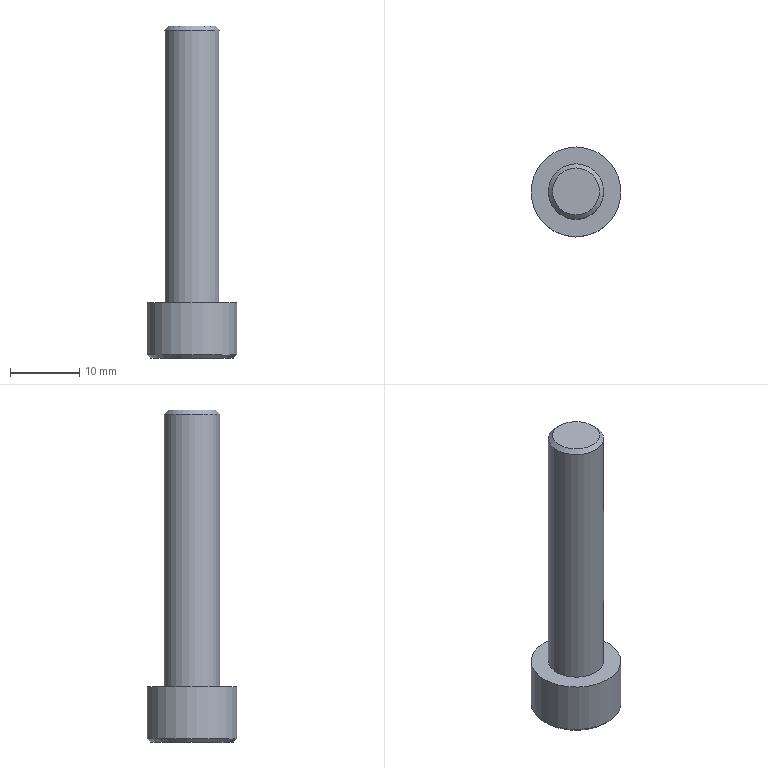Part | STEP file | gslz 2016.10.28-6_id226_x_t | 1 solid | 14 faces | box 13 x 13 x 48 mm | volume 2907 mm3 | plane 10 | cylinder 2 | cone 2 | commonest cylinder face diameters 8 x1 13 x1
STEP:
#1=CARTESIAN_POINT('',(-52.95,102.,99.992));
#2=VERTEX_POINT('',#1);
#3=CARTESIAN_POINT('',(-52.95,96.,99.992));
#4=DIRECTION('',(0.,0.,-1.));
#5=DIRECTION('',(0.,1.,0.));
#6=AXIS2_PLACEMENT_3D('',#3,#4,#5);
#7=CIRCLE('',#6,6.);
#8=EDGE_CURVE('',#2,#2,#7,.T.);
#9=ORIENTED_EDGE('',*,*,#8,.T.);
#10=EDGE_LOOP('',(#9));
#11=FACE_BOUND('',#10,.T.);
#12=CARTESIAN_POINT('',(-51.218,93.,99.992));
#13=VERTEX_POINT('',#12);
#14=CARTESIAN_POINT('',(-54.682,93.,99.992));
#15=VERTEX_POINT('',#14);
#16=CARTESIAN_POINT('',(-51.218,93.,99.992));
#17=DIRECTION('',(-1.,0.,0.));
#18=VECTOR('',#17,1.);
#19=LINE('',#16,#18);
#20=EDGE_CURVE('',#13,#15,#19,.T.);
#21=ORIENTED_EDGE('',*,*,#20,.F.);
#22=CARTESIAN_POINT('',(-49.486,96.,99.992));
#23=VERTEX_POINT('',#22);
#24=CARTESIAN_POINT('',(-49.486,96.,99.992));
#25=DIRECTION('',(-0.5,-0.866,0.));
#26=VECTOR('',#25,1.);
#27=LINE('',#24,#26);
#28=EDGE_CURVE('',#23,#13,#27,.T.);
#29=ORIENTED_EDGE('',*,*,#28,.F.);
#30=CARTESIAN_POINT('',(-51.218,99.,99.992));
#31=VERTEX_POINT('',#30);
#32=CARTESIAN_POINT('',(-51.218,99.,99.992));
#33=DIRECTION('',(0.5,-0.866,0.));
#34=VECTOR('',#33,1.);
#35=LINE('',#32,#34);
#36=EDGE_CURVE('',#31,#23,#35,.T.);
#37=ORIENTED_EDGE('',*,*,#36,.F.);
#38=CARTESIAN_POINT('',(-54.682,99.,99.992));
#39=VERTEX_POINT('',#38);
#40=CARTESIAN_POINT('',(-54.682,99.,99.992));
#41=DIRECTION('',(1.,0.,0.));
#42=VECTOR('',#41,1.);
#43=LINE('',#40,#42);
#44=EDGE_CURVE('',#39,#31,#43,.T.);
#45=ORIENTED_EDGE('',*,*,#44,.F.);
#46=CARTESIAN_POINT('',(-56.414,96.,99.992));
#47=VERTEX_POINT('',#46);
#48=CARTESIAN_POINT('',(-56.414,96.,99.992));
#49=DIRECTION('',(0.5,0.866,0.));
#50=VECTOR('',#49,1.);
#51=LINE('',#48,#50);
#52=EDGE_CURVE('',#47,#39,#51,.T.);
#53=ORIENTED_EDGE('',*,*,#52,.F.);
#54=CARTESIAN_POINT('',(-54.682,93.,99.992));
#55=DIRECTION('',(-0.5,0.866,0.));
#56=VECTOR('',#55,1.);
#57=LINE('',#54,#56);
#58=EDGE_CURVE('',#15,#47,#57,.T.);
#59=ORIENTED_EDGE('',*,*,#58,.F.);
#60=EDGE_LOOP('',(#21,#29,#37,#45,#53,#59));
#61=FACE_BOUND('',#60,.T.);
#62=CARTESIAN_POINT('',(-52.95,96.,99.992));
#63=DIRECTION('',(0.,0.,-1.));
#64=DIRECTION('',(0.,-1.,0.));
#65=AXIS2_PLACEMENT_3D('',#62,#63,#64);
#66=PLANE('',#65);
#67=ADVANCED_FACE('',(#11,#61),#66,.T.);
#68=CARTESIAN_POINT('',(-52.95,92.6,147.992));
#69=VERTEX_POINT('',#68);
#70=CARTESIAN_POINT('',(-52.95,96.,147.992));
#71=DIRECTION('',(0.,0.,1.));
#72=DIRECTION('',(0.,-1.,0.));
#73=AXIS2_PLACEMENT_3D('',#70,#71,#72);
#74=CIRCLE('',#73,3.4);
#75=EDGE_CURVE('',#69,#69,#74,.T.);
#76=ORIENTED_EDGE('',*,*,#75,.T.);
#77=EDGE_LOOP('',(#76));
#78=FACE_OUTER_BOUND('',#77,.T.);
#79=CARTESIAN_POINT('',(-52.95,96.,147.992));
#80=DIRECTION('',(0.,0.,1.));
#81=DIRECTION('',(0.,1.,0.));
#82=AXIS2_PLACEMENT_3D('',#79,#80,#81);
#83=PLANE('',#82);
#84=ADVANCED_FACE('',(#78),#83,.T.);
#85=CARTESIAN_POINT('',(-52.95,92.,147.392));
#86=VERTEX_POINT('',#85);
#87=CARTESIAN_POINT('',(-52.95,96.,147.392));
#88=DIRECTION('',(0.,0.,-1.));
#89=DIRECTION('',(0.,-1.,0.));
#90=AXIS2_PLACEMENT_3D('',#87,#88,#89);
#91=CIRCLE('',#90,4.);
#92=EDGE_CURVE('',#86,#86,#91,.T.);
#93=ORIENTED_EDGE('',*,*,#92,.T.);
#94=EDGE_LOOP('',(#93));
#95=FACE_BOUND('',#94,.T.);
#96=CARTESIAN_POINT('',(-52.95,92.,107.992));
#97=VERTEX_POINT('',#96);
#98=CARTESIAN_POINT('',(-52.95,96.,107.992));
#99=DIRECTION('',(0.,0.,1.));
#100=DIRECTION('',(0.,-1.,0.));
#101=AXIS2_PLACEMENT_3D('',#98,#99,#100);
#102=CIRCLE('',#101,4.);
#103=EDGE_CURVE('',#97,#97,#102,.T.);
#104=ORIENTED_EDGE('',*,*,#103,.T.);
#105=EDGE_LOOP('',(#104));
#106=FACE_BOUND('',#105,.T.);
#107=CARTESIAN_POINT('',(-52.95,96.,129.992));
#108=DIRECTION('',(0.,0.,1.));
#109=DIRECTION('',(1.,0.,0.));
#110=AXIS2_PLACEMENT_3D('',#107,#108,#109);
#111=CYLINDRICAL_SURFACE('',#110,4.);
#112=ADVANCED_FACE('',(#95,#106),#111,.T.);
#113=ORIENTED_EDGE('',*,*,#103,.F.);
#114=EDGE_LOOP('',(#113));
#115=FACE_BOUND('',#114,.T.);
#116=CARTESIAN_POINT('',(-52.95,89.5,107.992));
#117=VERTEX_POINT('',#116);
#118=CARTESIAN_POINT('',(-52.95,96.,107.992));
#119=DIRECTION('',(0.,0.,1.));
#120=DIRECTION('',(0.,-1.,0.));
#121=AXIS2_PLACEMENT_3D('',#118,#119,#120);
#122=CIRCLE('',#121,6.5);
#123=EDGE_CURVE('',#117,#117,#122,.T.);
#124=ORIENTED_EDGE('',*,*,#123,.T.);
#125=EDGE_LOOP('',(#124));
#126=FACE_BOUND('',#125,.T.);
#127=CARTESIAN_POINT('',(-52.95,96.,107.992));
#128=DIRECTION('',(0.,0.,1.));
#129=DIRECTION('',(0.,1.,0.));
#130=AXIS2_PLACEMENT_3D('',#127,#128,#129);
#131=PLANE('',#130);
#132=ADVANCED_FACE('',(#115,#126),#131,.T.);
#133=CARTESIAN_POINT('',(-52.95,102.5,100.492));
#134=VERTEX_POINT('',#133);
#135=CARTESIAN_POINT('',(-52.95,96.,100.492));
#136=DIRECTION('',(0.,0.,1.));
#137=DIRECTION('',(0.,1.,0.));
#138=AXIS2_PLACEMENT_3D('',#135,#136,#137);
#139=CIRCLE('',#138,6.5);
#140=EDGE_CURVE('',#134,#134,#139,.T.);
#141=ORIENTED_EDGE('',*,*,#140,.T.);
#142=EDGE_LOOP('',(#141));
#143=FACE_BOUND('',#142,.T.);
#144=ORIENTED_EDGE('',*,*,#123,.F.);
#145=EDGE_LOOP('',(#144));
#146=FACE_BOUND('',#145,.T.);
#147=CARTESIAN_POINT('',(-52.95,96.,96.992));
#148=DIRECTION('',(0.,0.,1.));
#149=DIRECTION('',(1.,0.,0.));
#150=AXIS2_PLACEMENT_3D('',#147,#148,#149);
#151=CYLINDRICAL_SURFACE('',#150,6.5);
#152=ADVANCED_FACE('',(#143,#146),#151,.T.);
#153=ORIENTED_EDGE('',*,*,#92,.F.);
#154=EDGE_LOOP('',(#153));
#155=FACE_BOUND('',#154,.T.);
#156=ORIENTED_EDGE('',*,*,#75,.F.);
#157=EDGE_LOOP('',(#156));
#158=FACE_BOUND('',#157,.T.);
#159=CARTESIAN_POINT('',(-52.95,96.,147.992));
#160=DIRECTION('',(0.,0.,-1.));
#161=DIRECTION('',(0.,1.,0.));
#162=AXIS2_PLACEMENT_3D('',#159,#160,#161);
#163=CONICAL_SURFACE('',#162,3.4,45.);
#164=ADVANCED_FACE('',(#155,#158),#163,.T.);
#165=ORIENTED_EDGE('',*,*,#20,.T.);
#166=CARTESIAN_POINT('',(-54.682,93.,104.992));
#167=VERTEX_POINT('',#166);
#168=CARTESIAN_POINT('',(-54.682,93.,104.992));
#169=DIRECTION('',(0.,0.,1.));
#170=VECTOR('',#169,1.);
#171=LINE('',#168,#170);
#172=EDGE_CURVE('',#15,#167,#171,.T.);
#173=ORIENTED_EDGE('',*,*,#172,.T.);
#174=CARTESIAN_POINT('',(-51.218,93.,104.992));
#175=VERTEX_POINT('',#174);
#176=CARTESIAN_POINT('',(-51.218,93.,104.992));
#177=DIRECTION('',(1.,0.,0.));
#178=VECTOR('',#177,1.);
#179=LINE('',#176,#178);
#180=EDGE_CURVE('',#167,#175,#179,.T.);
#181=ORIENTED_EDGE('',*,*,#180,.T.);
#182=CARTESIAN_POINT('',(-51.218,93.,104.992));
#183=DIRECTION('',(0.,0.,1.));
#184=VECTOR('',#183,1.);
#185=LINE('',#182,#184);
#186=EDGE_CURVE('',#13,#175,#185,.T.);
#187=ORIENTED_EDGE('',*,*,#186,.F.);
#188=EDGE_LOOP('',(#165,#173,#181,#187));
#189=FACE_OUTER_BOUND('',#188,.T.);
#190=CARTESIAN_POINT('',(-51.218,93.,104.992));
#191=DIRECTION('',(0.,-1.,0.));
#192=DIRECTION('',(0.,0.,-1.));
#193=AXIS2_PLACEMENT_3D('',#190,#191,#192);
#194=PLANE('',#193);
#195=ADVANCED_FACE('',(#189),#194,.F.);
#196=ORIENTED_EDGE('',*,*,#58,.T.);
#197=CARTESIAN_POINT('',(-56.414,96.,104.992));
#198=VERTEX_POINT('',#197);
#199=CARTESIAN_POINT('',(-56.414,96.,104.992));
#200=DIRECTION('',(0.,0.,1.));
#201=VECTOR('',#200,1.);
#202=LINE('',#199,#201);
#203=EDGE_CURVE('',#47,#198,#202,.T.);
#204=ORIENTED_EDGE('',*,*,#203,.T.);
#205=CARTESIAN_POINT('',(-54.682,93.,104.992));
#206=DIRECTION('',(0.5,-0.866,0.));
#207=VECTOR('',#206,1.);
#208=LINE('',#205,#207);
#209=EDGE_CURVE('',#198,#167,#208,.T.);
#210=ORIENTED_EDGE('',*,*,#209,.T.);
#211=ORIENTED_EDGE('',*,*,#172,.F.);
#212=EDGE_LOOP('',(#196,#204,#210,#211));
#213=FACE_OUTER_BOUND('',#212,.T.);
#214=CARTESIAN_POINT('',(-54.682,93.,104.992));
#215=DIRECTION('',(-0.866,-0.5,0.));
#216=DIRECTION('',(0.5,-0.866,0.));
#217=AXIS2_PLACEMENT_3D('',#214,#215,#216);
#218=PLANE('',#217);
#219=ADVANCED_FACE('',(#213),#218,.F.);
#220=ORIENTED_EDGE('',*,*,#52,.T.);
#221=CARTESIAN_POINT('',(-54.682,99.,104.992));
#222=VERTEX_POINT('',#221);
#223=CARTESIAN_POINT('',(-54.682,99.,104.992));
#224=DIRECTION('',(0.,0.,1.));
#225=VECTOR('',#224,1.);
#226=LINE('',#223,#225);
#227=EDGE_CURVE('',#39,#222,#226,.T.);
#228=ORIENTED_EDGE('',*,*,#227,.T.);
#229=CARTESIAN_POINT('',(-56.414,96.,104.992));
#230=DIRECTION('',(-0.5,-0.866,0.));
#231=VECTOR('',#230,1.);
#232=LINE('',#229,#231);
#233=EDGE_CURVE('',#222,#198,#232,.T.);
#234=ORIENTED_EDGE('',*,*,#233,.T.);
#235=ORIENTED_EDGE('',*,*,#203,.F.);
#236=EDGE_LOOP('',(#220,#228,#234,#235));
#237=FACE_OUTER_BOUND('',#236,.T.);
#238=CARTESIAN_POINT('',(-56.414,96.,104.992));
#239=DIRECTION('',(-0.866,0.5,0.));
#240=DIRECTION('',(-0.5,-0.866,0.));
#241=AXIS2_PLACEMENT_3D('',#238,#239,#240);
#242=PLANE('',#241);
#243=ADVANCED_FACE('',(#237),#242,.F.);
#244=ORIENTED_EDGE('',*,*,#44,.T.);
#245=CARTESIAN_POINT('',(-51.218,99.,104.992));
#246=VERTEX_POINT('',#245);
#247=CARTESIAN_POINT('',(-51.218,99.,104.992));
#248=DIRECTION('',(0.,0.,1.));
#249=VECTOR('',#248,1.);
#250=LINE('',#247,#249);
#251=EDGE_CURVE('',#31,#246,#250,.T.);
#252=ORIENTED_EDGE('',*,*,#251,.T.);
#253=CARTESIAN_POINT('',(-54.682,99.,104.992));
#254=DIRECTION('',(-1.,0.,0.));
#255=VECTOR('',#254,1.);
#256=LINE('',#253,#255);
#257=EDGE_CURVE('',#246,#222,#256,.T.);
#258=ORIENTED_EDGE('',*,*,#257,.T.);
#259=ORIENTED_EDGE('',*,*,#227,.F.);
#260=EDGE_LOOP('',(#244,#252,#258,#259));
#261=FACE_OUTER_BOUND('',#260,.T.);
#262=CARTESIAN_POINT('',(-54.682,99.,104.992));
#263=DIRECTION('',(0.,1.,0.));
#264=DIRECTION('',(0.,0.,-1.));
#265=AXIS2_PLACEMENT_3D('',#262,#263,#264);
#266=PLANE('',#265);
#267=ADVANCED_FACE('',(#261),#266,.F.);
#268=ORIENTED_EDGE('',*,*,#36,.T.);
#269=CARTESIAN_POINT('',(-49.486,96.,104.992));
#270=VERTEX_POINT('',#269);
#271=CARTESIAN_POINT('',(-49.486,96.,104.992));
#272=DIRECTION('',(0.,0.,1.));
#273=VECTOR('',#272,1.);
#274=LINE('',#271,#273);
#275=EDGE_CURVE('',#23,#270,#274,.T.);
#276=ORIENTED_EDGE('',*,*,#275,.T.);
#277=CARTESIAN_POINT('',(-51.218,99.,104.992));
#278=DIRECTION('',(-0.5,0.866,0.));
#279=VECTOR('',#278,1.);
#280=LINE('',#277,#279);
#281=EDGE_CURVE('',#270,#246,#280,.T.);
#282=ORIENTED_EDGE('',*,*,#281,.T.);
#283=ORIENTED_EDGE('',*,*,#251,.F.);
#284=EDGE_LOOP('',(#268,#276,#282,#283));
#285=FACE_OUTER_BOUND('',#284,.T.);
#286=CARTESIAN_POINT('',(-51.218,99.,104.992));
#287=DIRECTION('',(0.866,0.5,0.));
#288=DIRECTION('',(-0.5,0.866,0.));
#289=AXIS2_PLACEMENT_3D('',#286,#287,#288);
#290=PLANE('',#289);
#291=ADVANCED_FACE('',(#285),#290,.F.);
#292=ORIENTED_EDGE('',*,*,#28,.T.);
#293=ORIENTED_EDGE('',*,*,#186,.T.);
#294=CARTESIAN_POINT('',(-49.486,96.,104.992));
#295=DIRECTION('',(0.5,0.866,0.));
#296=VECTOR('',#295,1.);
#297=LINE('',#294,#296);
#298=EDGE_CURVE('',#175,#270,#297,.T.);
#299=ORIENTED_EDGE('',*,*,#298,.T.);
#300=ORIENTED_EDGE('',*,*,#275,.F.);
#301=EDGE_LOOP('',(#292,#293,#299,#300));
#302=FACE_OUTER_BOUND('',#301,.T.);
#303=CARTESIAN_POINT('',(-49.486,96.,104.992));
#304=DIRECTION('',(0.866,-0.5,0.));
#305=DIRECTION('',(0.5,0.866,0.));
#306=AXIS2_PLACEMENT_3D('',#303,#304,#305);
#307=PLANE('',#306);
#308=ADVANCED_FACE('',(#302),#307,.F.);
#309=ORIENTED_EDGE('',*,*,#180,.F.);
#310=ORIENTED_EDGE('',*,*,#209,.F.);
#311=ORIENTED_EDGE('',*,*,#233,.F.);
#312=ORIENTED_EDGE('',*,*,#257,.F.);
#313=ORIENTED_EDGE('',*,*,#281,.F.);
#314=ORIENTED_EDGE('',*,*,#298,.F.);
#315=EDGE_LOOP('',(#309,#310,#311,#312,#313,#314));
#316=FACE_OUTER_BOUND('',#315,.T.);
#317=CARTESIAN_POINT('',(-54.682,93.,104.992));
#318=DIRECTION('',(0.,0.,-1.));
#319=DIRECTION('',(0.,-1.,0.));
#320=AXIS2_PLACEMENT_3D('',#317,#318,#319);
#321=PLANE('',#320);
#322=ADVANCED_FACE('',(#316),#321,.T.);
#323=ORIENTED_EDGE('',*,*,#8,.F.);
#324=EDGE_LOOP('',(#323));
#325=FACE_BOUND('',#324,.T.);
#326=ORIENTED_EDGE('',*,*,#140,.F.);
#327=EDGE_LOOP('',(#326));
#328=FACE_BOUND('',#327,.T.);
#329=CARTESIAN_POINT('',(-52.95,96.,100.492));
#330=DIRECTION('',(0.,0.,1.));
#331=DIRECTION('',(1.,0.,0.));
#332=AXIS2_PLACEMENT_3D('',#329,#330,#331);
#333=CONICAL_SURFACE('',#332,6.5,45.);
#334=ADVANCED_FACE('',(#325,#328),#333,.T.);
#335=CLOSED_SHELL('',(#67,#84,#112,#132,#152,#164,#195,#219,#243,#267,#291,#308,#322,#334));
#336=MANIFOLD_SOLID_BREP('',#335);
#337=(LENGTH_UNIT()NAMED_UNIT(*)SI_UNIT(.MILLI.,.METRE.));
#338=UNCERTAINTY_MEASURE_WITH_UNIT(LENGTH_MEASURE(0.00002),#337,'','');
#339=(NAMED_UNIT(*)PLANE_ANGLE_UNIT()SI_UNIT($,.RADIAN.));
#340=PLANE_ANGLE_MEASURE_WITH_UNIT(PLANE_ANGLE_MEASURE(0.01745),#339);
#341=DIMENSIONAL_EXPONENTS(0.,0.,0.,0.,0.,0.,0.);
#342=(CONVERSION_BASED_UNIT('DEGREE',#340)NAMED_UNIT(#341)PLANE_ANGLE_UNIT());
#343=(NAMED_UNIT(*)SI_UNIT($,.STERADIAN.)SOLID_ANGLE_UNIT());
#344=(GEOMETRIC_REPRESENTATION_CONTEXT(3)GLOBAL_UNCERTAINTY_ASSIGNED_CONTEXT((#338))GLOBAL_UNIT_ASSIGNED_CONTEXT((#337,#342,#343))REPRESENTATION_CONTEXT('',''));
#345=ADVANCED_BREP_SHAPE_REPRESENTATION('',(#336),#344);